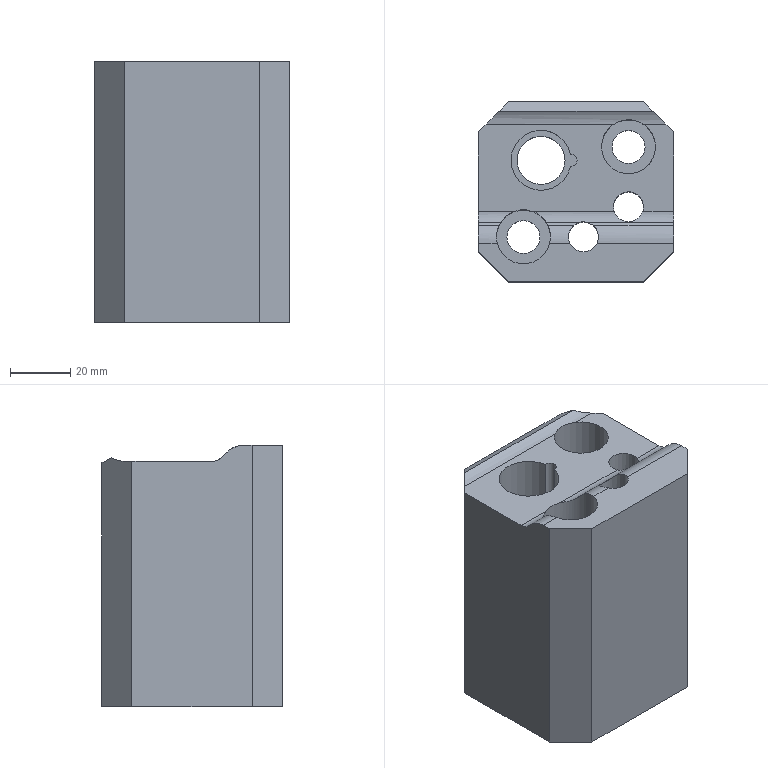Part | NX | features solid 2 | 1 solid | 35 faces | box 65 x 60 x 87.008 mm | volume 234340 mm3 | plane 19 | cylinder 16 | commonest cylinder face diameters 16 x5 10 x4 11 x2 18 x2 4 x1 20 x1
STEP:
#1=CARTESIAN_POINT('',(-255.,-515.,5.));
#2=VERTEX_POINT('',#1);
#3=CARTESIAN_POINT('',(-255.,-515.,92.008));
#4=VERTEX_POINT('',#3);
#5=CARTESIAN_POINT('',(-255.,-515.,10.));
#6=DIRECTION('',(0.,0.,1.));
#7=VECTOR('',#6,1000.);
#8=LINE('',#5,#7);
#9=EDGE_CURVE('',#2,#4,#8,.T.);
#10=ORIENTED_EDGE('',*,*,#9,.T.);
#11=CARTESIAN_POINT('',(-300.,-515.,92.008));
#12=VERTEX_POINT('',#11);
#13=CARTESIAN_POINT('',(-260.,-515.,92.008));
#14=DIRECTION('',(-1.,0.,0.));
#15=VECTOR('',#14,1000.);
#16=LINE('',#13,#15);
#17=EDGE_CURVE('',#4,#12,#16,.T.);
#18=ORIENTED_EDGE('',*,*,#17,.T.);
#19=CARTESIAN_POINT('',(-300.,-515.,5.));
#20=VERTEX_POINT('',#19);
#21=CARTESIAN_POINT('',(-300.,-515.,10.));
#22=DIRECTION('',(0.,0.,-1.));
#23=VECTOR('',#22,1000.);
#24=LINE('',#21,#23);
#25=EDGE_CURVE('',#12,#20,#24,.T.);
#26=ORIENTED_EDGE('',*,*,#25,.T.);
#27=CARTESIAN_POINT('',(-260.,-515.,5.));
#28=DIRECTION('',(1.,0.,0.));
#29=VECTOR('',#28,1000.);
#30=LINE('',#27,#29);
#31=EDGE_CURVE('',#20,#2,#30,.T.);
#32=ORIENTED_EDGE('',*,*,#31,.T.);
#33=EDGE_LOOP('',(#10,#18,#26,#32));
#34=FACE_BOUND('',#33,.T.);
#35=CARTESIAN_POINT('',(-260.,-515.,10.));
#36=DIRECTION('',(0.,-1.,0.));
#37=DIRECTION('',(0.,0.,-1.));
#38=AXIS2_PLACEMENT_3D('',#35,#36,#37);
#39=PLANE('',#38);
#40=ADVANCED_FACE('',(#34),#39,.T.);
#41=CARTESIAN_POINT('',(-310.,-505.,5.));
#42=VERTEX_POINT('',#41);
#43=CARTESIAN_POINT('',(-310.,-505.,92.008));
#44=VERTEX_POINT('',#43);
#45=CARTESIAN_POINT('',(-310.,-505.,10.));
#46=DIRECTION('',(0.,0.,1.));
#47=VECTOR('',#46,1000.);
#48=LINE('',#45,#47);
#49=EDGE_CURVE('',#42,#44,#48,.T.);
#50=ORIENTED_EDGE('',*,*,#49,.T.);
#51=CARTESIAN_POINT('',(-310.,-502.176,92.008));
#52=VERTEX_POINT('',#51);
#53=CARTESIAN_POINT('',(-310.,-505.,92.008));
#54=DIRECTION('',(0.,1.,0.));
#55=VECTOR('',#54,1000.);
#56=LINE('',#53,#55);
#57=EDGE_CURVE('',#44,#52,#56,.T.);
#58=ORIENTED_EDGE('',*,*,#57,.T.);
#59=CARTESIAN_POINT('',(-310.,-496.288,89.423));
#60=VERTEX_POINT('',#59);
#61=CARTESIAN_POINT('',(-310.,-502.176,84.008));
#62=DIRECTION('',(-1.,0.,0.));
#63=DIRECTION('',(0.,0.,1.));
#64=AXIS2_PLACEMENT_3D('',#61,#62,#63);
#65=CIRCLE('',#64,8.);
#66=EDGE_CURVE('',#52,#60,#65,.T.);
#67=ORIENTED_EDGE('',*,*,#66,.T.);
#68=CARTESIAN_POINT('',(-310.,-495.276,88.323));
#69=VERTEX_POINT('',#68);
#70=CARTESIAN_POINT('',(-310.,-460.707,50.738));
#71=DIRECTION('',(0.,0.677,-0.736));
#72=VECTOR('',#71,1000.);
#73=LINE('',#70,#72);
#74=EDGE_CURVE('',#60,#69,#73,.T.);
#75=ORIENTED_EDGE('',*,*,#74,.T.);
#76=CARTESIAN_POINT('',(-310.,-491.596,86.708));
#77=VERTEX_POINT('',#76);
#78=CARTESIAN_POINT('',(-310.,-491.596,91.708));
#79=DIRECTION('',(-1.,0.,0.));
#80=DIRECTION('',(0.,0.,1.));
#81=AXIS2_PLACEMENT_3D('',#78,#79,#80);
#82=CIRCLE('',#81,5.);
#83=EDGE_CURVE('',#77,#69,#82,.T.);
#84=ORIENTED_EDGE('',*,*,#83,.F.);
#85=CARTESIAN_POINT('',(-310.,-465.,86.708));
#86=VERTEX_POINT('',#85);
#87=CARTESIAN_POINT('',(-310.,-505.,86.708));
#88=DIRECTION('',(0.,1.,0.));
#89=VECTOR('',#88,1000.);
#90=LINE('',#87,#89);
#91=EDGE_CURVE('',#77,#86,#90,.T.);
#92=ORIENTED_EDGE('',*,*,#91,.T.);
#93=CARTESIAN_POINT('',(-310.,-465.,5.));
#94=VERTEX_POINT('',#93);
#95=CARTESIAN_POINT('',(-310.,-465.,10.));
#96=DIRECTION('',(0.,0.,-1.));
#97=VECTOR('',#96,1000.);
#98=LINE('',#95,#97);
#99=EDGE_CURVE('',#86,#94,#98,.T.);
#100=ORIENTED_EDGE('',*,*,#99,.T.);
#101=CARTESIAN_POINT('',(-310.,-505.,5.));
#102=DIRECTION('',(0.,-1.,0.));
#103=VECTOR('',#102,1000.);
#104=LINE('',#101,#103);
#105=EDGE_CURVE('',#94,#42,#104,.T.);
#106=ORIENTED_EDGE('',*,*,#105,.T.);
#107=EDGE_LOOP('',(#50,#58,#67,#75,#84,#92,#100,#106));
#108=FACE_BOUND('',#107,.T.);
#109=CARTESIAN_POINT('',(-310.,-505.,10.));
#110=DIRECTION('',(-1.,0.,0.));
#111=DIRECTION('',(0.,0.,1.));
#112=AXIS2_PLACEMENT_3D('',#109,#110,#111);
#113=PLANE('',#112);
#114=ADVANCED_FACE('',(#108),#113,.T.);
#115=CARTESIAN_POINT('',(-300.,-455.,5.));
#116=VERTEX_POINT('',#115);
#117=CARTESIAN_POINT('',(-300.,-455.,86.231));
#118=VERTEX_POINT('',#117);
#119=CARTESIAN_POINT('',(-300.,-455.,10.));
#120=DIRECTION('',(0.,0.,1.));
#121=VECTOR('',#120,1000.);
#122=LINE('',#119,#121);
#123=EDGE_CURVE('',#116,#118,#122,.T.);
#124=ORIENTED_EDGE('',*,*,#123,.T.);
#125=CARTESIAN_POINT('',(-255.,-455.,86.231));
#126=VERTEX_POINT('',#125);
#127=CARTESIAN_POINT('',(-255.,-455.,86.231));
#128=DIRECTION('',(1.,0.,0.));
#129=VECTOR('',#128,1000.);
#130=LINE('',#127,#129);
#131=EDGE_CURVE('',#118,#126,#130,.T.);
#132=ORIENTED_EDGE('',*,*,#131,.T.);
#133=CARTESIAN_POINT('',(-255.,-455.,5.));
#134=VERTEX_POINT('',#133);
#135=CARTESIAN_POINT('',(-255.,-455.,10.));
#136=DIRECTION('',(0.,0.,-1.));
#137=VECTOR('',#136,1000.);
#138=LINE('',#135,#137);
#139=EDGE_CURVE('',#126,#134,#138,.T.);
#140=ORIENTED_EDGE('',*,*,#139,.T.);
#141=CARTESIAN_POINT('',(-260.,-455.,5.));
#142=DIRECTION('',(-1.,0.,0.));
#143=VECTOR('',#142,1000.);
#144=LINE('',#141,#143);
#145=EDGE_CURVE('',#134,#116,#144,.T.);
#146=ORIENTED_EDGE('',*,*,#145,.T.);
#147=EDGE_LOOP('',(#124,#132,#140,#146));
#148=FACE_BOUND('',#147,.T.);
#149=CARTESIAN_POINT('',(-260.,-455.,10.));
#150=DIRECTION('',(0.,1.,0.));
#151=DIRECTION('',(0.,0.,1.));
#152=AXIS2_PLACEMENT_3D('',#149,#150,#151);
#153=PLANE('',#152);
#154=ADVANCED_FACE('',(#148),#153,.T.);
#155=CARTESIAN_POINT('',(-245.,-496.288,89.423));
#156=VERTEX_POINT('',#155);
#157=CARTESIAN_POINT('',(-245.,-502.176,92.008));
#158=VERTEX_POINT('',#157);
#159=CARTESIAN_POINT('',(-245.,-502.176,84.008));
#160=DIRECTION('',(1.,0.,0.));
#161=DIRECTION('',(0.,0.,-1.));
#162=AXIS2_PLACEMENT_3D('',#159,#160,#161);
#163=CIRCLE('',#162,8.);
#164=EDGE_CURVE('',#156,#158,#163,.T.);
#165=ORIENTED_EDGE('',*,*,#164,.T.);
#166=CARTESIAN_POINT('',(-245.,-505.,92.008));
#167=VERTEX_POINT('',#166);
#168=CARTESIAN_POINT('',(-245.,-505.,92.008));
#169=DIRECTION('',(0.,-1.,0.));
#170=VECTOR('',#169,1000.);
#171=LINE('',#168,#170);
#172=EDGE_CURVE('',#158,#167,#171,.T.);
#173=ORIENTED_EDGE('',*,*,#172,.T.);
#174=CARTESIAN_POINT('',(-245.,-505.,5.));
#175=VERTEX_POINT('',#174);
#176=CARTESIAN_POINT('',(-245.,-505.,10.));
#177=DIRECTION('',(0.,0.,-1.));
#178=VECTOR('',#177,1000.);
#179=LINE('',#176,#178);
#180=EDGE_CURVE('',#167,#175,#179,.T.);
#181=ORIENTED_EDGE('',*,*,#180,.T.);
#182=CARTESIAN_POINT('',(-245.,-465.,5.));
#183=VERTEX_POINT('',#182);
#184=CARTESIAN_POINT('',(-245.,-505.,5.));
#185=DIRECTION('',(0.,1.,0.));
#186=VECTOR('',#185,1000.);
#187=LINE('',#184,#186);
#188=EDGE_CURVE('',#175,#183,#187,.T.);
#189=ORIENTED_EDGE('',*,*,#188,.T.);
#190=CARTESIAN_POINT('',(-245.,-465.,86.708));
#191=VERTEX_POINT('',#190);
#192=CARTESIAN_POINT('',(-245.,-465.,10.));
#193=DIRECTION('',(0.,0.,1.));
#194=VECTOR('',#193,1000.);
#195=LINE('',#192,#194);
#196=EDGE_CURVE('',#183,#191,#195,.T.);
#197=ORIENTED_EDGE('',*,*,#196,.T.);
#198=CARTESIAN_POINT('',(-245.,-491.596,86.708));
#199=VERTEX_POINT('',#198);
#200=CARTESIAN_POINT('',(-245.,-505.,86.708));
#201=DIRECTION('',(0.,-1.,0.));
#202=VECTOR('',#201,1000.);
#203=LINE('',#200,#202);
#204=EDGE_CURVE('',#191,#199,#203,.T.);
#205=ORIENTED_EDGE('',*,*,#204,.T.);
#206=CARTESIAN_POINT('',(-245.,-495.276,88.323));
#207=VERTEX_POINT('',#206);
#208=CARTESIAN_POINT('',(-245.,-491.596,91.708));
#209=DIRECTION('',(1.,0.,0.));
#210=DIRECTION('',(0.,0.,-1.));
#211=AXIS2_PLACEMENT_3D('',#208,#209,#210);
#212=CIRCLE('',#211,5.);
#213=EDGE_CURVE('',#207,#199,#212,.T.);
#214=ORIENTED_EDGE('',*,*,#213,.F.);
#215=CARTESIAN_POINT('',(-245.,-460.707,50.738));
#216=DIRECTION('',(0.,-0.677,0.736));
#217=VECTOR('',#216,1000.);
#218=LINE('',#215,#217);
#219=EDGE_CURVE('',#207,#156,#218,.T.);
#220=ORIENTED_EDGE('',*,*,#219,.T.);
#221=EDGE_LOOP('',(#165,#173,#181,#189,#197,#205,#214,#220));
#222=FACE_BOUND('',#221,.T.);
#223=CARTESIAN_POINT('',(-245.,-505.,10.));
#224=DIRECTION('',(1.,0.,0.));
#225=DIRECTION('',(0.,0.,-1.));
#226=AXIS2_PLACEMENT_3D('',#223,#224,#225);
#227=PLANE('',#226);
#228=ADVANCED_FACE('',(#222),#227,.T.);
#229=ORIENTED_EDGE('',*,*,#180,.F.);
#230=CARTESIAN_POINT('',(-255.,-515.,92.008));
#231=DIRECTION('',(0.7071,0.7071,0.));
#232=VECTOR('',#231,1000.);
#233=LINE('',#230,#232);
#234=EDGE_CURVE('',#167,#4,#233,.F.);
#235=ORIENTED_EDGE('',*,*,#234,.T.);
#236=ORIENTED_EDGE('',*,*,#9,.F.);
#237=CARTESIAN_POINT('',(-252.5,-512.5,5.));
#238=DIRECTION('',(0.7071,0.7071,0.));
#239=VECTOR('',#238,1000.);
#240=LINE('',#237,#239);
#241=EDGE_CURVE('',#175,#2,#240,.F.);
#242=ORIENTED_EDGE('',*,*,#241,.F.);
#243=EDGE_LOOP('',(#229,#235,#236,#242));
#244=FACE_BOUND('',#243,.T.);
#245=CARTESIAN_POINT('',(-255.,-515.,10.));
#246=DIRECTION('',(-0.7071,0.7071,0.));
#247=DIRECTION('',(-0.7071,-0.7071,0.));
#248=AXIS2_PLACEMENT_3D('',#245,#246,#247);
#249=PLANE('',#248);
#250=ADVANCED_FACE('',(#244),#249,.F.);
#251=ORIENTED_EDGE('',*,*,#25,.F.);
#252=CARTESIAN_POINT('',(-310.,-505.,92.008));
#253=DIRECTION('',(0.7071,-0.7071,0.));
#254=VECTOR('',#253,1000.);
#255=LINE('',#252,#254);
#256=EDGE_CURVE('',#12,#44,#255,.F.);
#257=ORIENTED_EDGE('',*,*,#256,.T.);
#258=ORIENTED_EDGE('',*,*,#49,.F.);
#259=CARTESIAN_POINT('',(-285.,-530.,5.));
#260=DIRECTION('',(0.7071,-0.7071,0.));
#261=VECTOR('',#260,1000.);
#262=LINE('',#259,#261);
#263=EDGE_CURVE('',#20,#42,#262,.F.);
#264=ORIENTED_EDGE('',*,*,#263,.F.);
#265=EDGE_LOOP('',(#251,#257,#258,#264));
#266=FACE_BOUND('',#265,.T.);
#267=CARTESIAN_POINT('',(-310.,-505.,10.));
#268=DIRECTION('',(0.7071,0.7071,0.));
#269=DIRECTION('',(-0.7071,0.7071,0.));
#270=AXIS2_PLACEMENT_3D('',#267,#268,#269);
#271=PLANE('',#270);
#272=ADVANCED_FACE('',(#266),#271,.F.);
#273=CARTESIAN_POINT('',(-303.154,-458.154,87.961));
#274=VERTEX_POINT('',#273);
#275=CARTESIAN_POINT('',(-307.454,-462.454,86.708));
#276=VERTEX_POINT('',#275);
#277=CARTESIAN_POINT('',(-307.454,-462.454,94.708));
#278=DIRECTION('',(0.7071,-0.7071,0.));
#279=DIRECTION('',(0.7071,0.7071,0.));
#280=AXIS2_PLACEMENT_3D('',#277,#278,#279);
#281=ELLIPSE('',#280,11.314,8.);
#282=EDGE_CURVE('',#274,#276,#281,.F.);
#283=ORIENTED_EDGE('',*,*,#282,.F.);
#284=CARTESIAN_POINT('',(-281.828,-436.828,76.264));
#285=DIRECTION('',(0.6593,0.6593,-0.3616));
#286=VECTOR('',#285,1000.);
#287=LINE('',#284,#286);
#288=EDGE_CURVE('',#274,#118,#287,.T.);
#289=ORIENTED_EDGE('',*,*,#288,.T.);
#290=ORIENTED_EDGE('',*,*,#123,.F.);
#291=CARTESIAN_POINT('',(-305.,-460.,5.));
#292=DIRECTION('',(-0.7071,-0.7071,0.));
#293=VECTOR('',#292,1000.);
#294=LINE('',#291,#293);
#295=EDGE_CURVE('',#94,#116,#294,.F.);
#296=ORIENTED_EDGE('',*,*,#295,.F.);
#297=ORIENTED_EDGE('',*,*,#99,.F.);
#298=CARTESIAN_POINT('',(-300.,-455.,86.708));
#299=DIRECTION('',(-0.7071,-0.7071,0.));
#300=VECTOR('',#299,1000.);
#301=LINE('',#298,#300);
#302=EDGE_CURVE('',#86,#276,#301,.F.);
#303=ORIENTED_EDGE('',*,*,#302,.T.);
#304=EDGE_LOOP('',(#283,#289,#290,#296,#297,#303));
#305=FACE_BOUND('',#304,.T.);
#306=CARTESIAN_POINT('',(-300.,-455.,10.));
#307=DIRECTION('',(0.7071,-0.7071,0.));
#308=DIRECTION('',(0.7071,0.7071,0.));
#309=AXIS2_PLACEMENT_3D('',#306,#307,#308);
#310=PLANE('',#309);
#311=ADVANCED_FACE('',(#305),#310,.F.);
#312=ORIENTED_EDGE('',*,*,#139,.F.);
#313=CARTESIAN_POINT('',(-251.846,-458.154,87.961));
#314=VERTEX_POINT('',#313);
#315=CARTESIAN_POINT('',(-264.48,-445.52,81.032));
#316=DIRECTION('',(0.6593,-0.6593,0.3616));
#317=VECTOR('',#316,1000.);
#318=LINE('',#315,#317);
#319=EDGE_CURVE('',#126,#314,#318,.T.);
#320=ORIENTED_EDGE('',*,*,#319,.T.);
#321=CARTESIAN_POINT('',(-247.546,-462.454,86.708));
#322=VERTEX_POINT('',#321);
#323=CARTESIAN_POINT('',(-247.546,-462.454,94.708));
#324=DIRECTION('',(-0.7071,-0.7071,0.));
#325=DIRECTION('',(0.7071,-0.7071,0.));
#326=AXIS2_PLACEMENT_3D('',#323,#324,#325);
#327=ELLIPSE('',#326,11.314,8.);
#328=EDGE_CURVE('',#322,#314,#327,.F.);
#329=ORIENTED_EDGE('',*,*,#328,.F.);
#330=CARTESIAN_POINT('',(-245.,-465.,86.708));
#331=DIRECTION('',(-0.7071,0.7071,0.));
#332=VECTOR('',#331,1000.);
#333=LINE('',#330,#332);
#334=EDGE_CURVE('',#322,#191,#333,.F.);
#335=ORIENTED_EDGE('',*,*,#334,.T.);
#336=ORIENTED_EDGE('',*,*,#196,.F.);
#337=CARTESIAN_POINT('',(-232.5,-477.5,5.));
#338=DIRECTION('',(-0.7071,0.7071,0.));
#339=VECTOR('',#338,1000.);
#340=LINE('',#337,#339);
#341=EDGE_CURVE('',#134,#183,#340,.F.);
#342=ORIENTED_EDGE('',*,*,#341,.F.);
#343=EDGE_LOOP('',(#312,#320,#329,#335,#336,#342));
#344=FACE_BOUND('',#343,.T.);
#345=CARTESIAN_POINT('',(-245.,-465.,10.));
#346=DIRECTION('',(-0.7071,-0.7071,0.));
#347=DIRECTION('',(0.7071,-0.7071,0.));
#348=AXIS2_PLACEMENT_3D('',#345,#346,#347);
#349=PLANE('',#348);
#350=ADVANCED_FACE('',(#344),#349,.F.);
#351=CARTESIAN_POINT('',(-269.,-470.,35.));
#352=VERTEX_POINT('',#351);
#353=CARTESIAN_POINT('',(-260.,-470.,35.));
#354=DIRECTION('',(0.,0.,-1.));
#355=DIRECTION('',(-1.,0.,0.));
#356=AXIS2_PLACEMENT_3D('',#353,#354,#355);
#357=CIRCLE('',#356,9.);
#358=EDGE_CURVE('',#352,#352,#357,.T.);
#359=ORIENTED_EDGE('',*,*,#358,.T.);
#360=EDGE_LOOP('',(#359));
#361=FACE_BOUND('',#360,.T.);
#362=CARTESIAN_POINT('',(-255.095,-462.454,86.708));
#363=VERTEX_POINT('',#362);
#364=CARTESIAN_POINT('',(-264.905,-462.454,86.708));
#365=VERTEX_POINT('',#364);
#366=CARTESIAN_POINT('',(-260.,-470.,86.708));
#367=DIRECTION('',(0.,0.,1.));
#368=DIRECTION('',(1.,0.,0.));
#369=AXIS2_PLACEMENT_3D('',#366,#367,#368);
#370=CIRCLE('',#369,9.);
#371=EDGE_CURVE('',#363,#365,#370,.F.);
#372=ORIENTED_EDGE('',*,*,#371,.F.);
#373=CARTESIAN_POINT('',(-255.095,-462.454,86.708));
#374=CARTESIAN_POINT('',(-256.558,-461.503,86.708));
#375=CARTESIAN_POINT('',(-259.984,-460.497,86.974));
#376=CARTESIAN_POINT('',(-263.442,-461.503,86.708));
#377=CARTESIAN_POINT('',(-264.905,-462.454,86.708));
#378=B_SPLINE_CURVE_WITH_KNOTS('',3,(#373,#374,#375,#376,#377),.UNSPECIFIED.,.F.,.F.,(4,1,4),(0.,0.00516,0.01032),.UNSPECIFIED.);
#379=EDGE_CURVE('',#363,#365,#378,.T.);
#380=ORIENTED_EDGE('',*,*,#379,.T.);
#381=EDGE_LOOP('',(#372,#380));
#382=FACE_BOUND('',#381,.T.);
#383=CARTESIAN_POINT('',(-260.,-470.,110.));
#384=DIRECTION('',(0.,0.,-1.));
#385=DIRECTION('',(-1.,0.,0.));
#386=AXIS2_PLACEMENT_3D('',#383,#384,#385);
#387=CYLINDRICAL_SURFACE('',#386,9.);
#388=ADVANCED_FACE('',(#361,#382),#387,.F.);
#389=CARTESIAN_POINT('',(-304.,-500.,35.));
#390=VERTEX_POINT('',#389);
#391=CARTESIAN_POINT('',(-295.,-500.,35.));
#392=DIRECTION('',(0.,0.,-1.));
#393=DIRECTION('',(-1.,0.,0.));
#394=AXIS2_PLACEMENT_3D('',#391,#392,#393);
#395=CIRCLE('',#394,9.);
#396=EDGE_CURVE('',#390,#390,#395,.T.);
#397=ORIENTED_EDGE('',*,*,#396,.T.);
#398=EDGE_LOOP('',(#397));
#399=FACE_BOUND('',#398,.T.);
#400=CARTESIAN_POINT('',(-286.801,-496.288,89.423));
#401=VERTEX_POINT('',#400);
#402=CARTESIAN_POINT('',(-286.267,-502.176,92.008));
#403=VERTEX_POINT('',#402);
#404=CARTESIAN_POINT('',(-286.801,-496.288,89.423));
#405=CARTESIAN_POINT('',(-286.47,-497.019,90.218));
#406=CARTESIAN_POINT('',(-285.896,-498.815,91.527));
#407=CARTESIAN_POINT('',(-285.993,-501.076,92.008));
#408=CARTESIAN_POINT('',(-286.267,-502.176,92.008));
#409=B_SPLINE_CURVE_WITH_KNOTS('',3,(#404,#405,#406,#407,#408),.UNSPECIFIED.,.F.,.F.,(4,1,4),(0.,0.00335,0.0067),.UNSPECIFIED.);
#410=EDGE_CURVE('',#401,#403,#409,.T.);
#411=ORIENTED_EDGE('',*,*,#410,.F.);
#412=CARTESIAN_POINT('',(-287.34,-495.276,88.323));
#413=VERTEX_POINT('',#412);
#414=CARTESIAN_POINT('',(-295.,-500.,93.459));
#415=DIRECTION('',(0.,0.736,0.677));
#416=DIRECTION('',(0.,0.677,-0.736));
#417=AXIS2_PLACEMENT_3D('',#414,#415,#416);
#418=ELLIPSE('',#417,13.295,9.);
#419=EDGE_CURVE('',#413,#401,#418,.F.);
#420=ORIENTED_EDGE('',*,*,#419,.F.);
#421=CARTESIAN_POINT('',(-291.78,-491.596,86.708));
#422=VERTEX_POINT('',#421);
#423=CARTESIAN_POINT('',(-287.34,-495.276,88.323));
#424=CARTESIAN_POINT('',(-287.745,-494.619,87.609));
#425=CARTESIAN_POINT('',(-288.986,-493.061,86.771));
#426=CARTESIAN_POINT('',(-290.803,-491.97,86.708));
#427=CARTESIAN_POINT('',(-291.78,-491.596,86.708));
#428=B_SPLINE_CURVE_WITH_KNOTS('',3,(#423,#424,#425,#426,#427),.UNSPECIFIED.,.F.,.F.,(4,1,4),(0.,0.003104,0.006208),.UNSPECIFIED.);
#429=EDGE_CURVE('',#413,#422,#428,.T.);
#430=ORIENTED_EDGE('',*,*,#429,.T.);
#431=CARTESIAN_POINT('',(-298.22,-491.596,86.708));
#432=VERTEX_POINT('',#431);
#433=CARTESIAN_POINT('',(-295.,-500.,86.708));
#434=DIRECTION('',(0.,0.,1.));
#435=DIRECTION('',(1.,0.,0.));
#436=AXIS2_PLACEMENT_3D('',#433,#434,#435);
#437=CIRCLE('',#436,9.);
#438=EDGE_CURVE('',#432,#422,#437,.F.);
#439=ORIENTED_EDGE('',*,*,#438,.F.);
#440=CARTESIAN_POINT('',(-302.66,-495.276,88.323));
#441=VERTEX_POINT('',#440);
#442=CARTESIAN_POINT('',(-298.22,-491.596,86.708));
#443=CARTESIAN_POINT('',(-299.198,-491.97,86.708));
#444=CARTESIAN_POINT('',(-301.015,-493.063,86.772));
#445=CARTESIAN_POINT('',(-302.255,-494.618,87.608));
#446=CARTESIAN_POINT('',(-302.66,-495.276,88.323));
#447=B_SPLINE_CURVE_WITH_KNOTS('',3,(#442,#443,#444,#445,#446),.UNSPECIFIED.,.F.,.F.,(4,1,4),(0.,0.003103,0.006207),.UNSPECIFIED.);
#448=EDGE_CURVE('',#432,#441,#447,.T.);
#449=ORIENTED_EDGE('',*,*,#448,.T.);
#450=CARTESIAN_POINT('',(-303.199,-496.288,89.423));
#451=VERTEX_POINT('',#450);
#452=CARTESIAN_POINT('',(-295.,-500.,93.459));
#453=DIRECTION('',(0.,0.736,0.677));
#454=DIRECTION('',(0.,0.677,-0.736));
#455=AXIS2_PLACEMENT_3D('',#452,#453,#454);
#456=ELLIPSE('',#455,13.295,9.);
#457=EDGE_CURVE('',#451,#441,#456,.F.);
#458=ORIENTED_EDGE('',*,*,#457,.F.);
#459=CARTESIAN_POINT('',(-303.733,-502.176,92.008));
#460=VERTEX_POINT('',#459);
#461=CARTESIAN_POINT('',(-303.733,-502.176,92.008));
#462=CARTESIAN_POINT('',(-304.007,-501.078,92.008));
#463=CARTESIAN_POINT('',(-304.105,-498.822,91.531));
#464=CARTESIAN_POINT('',(-303.53,-497.019,90.218));
#465=CARTESIAN_POINT('',(-303.199,-496.288,89.423));
#466=B_SPLINE_CURVE_WITH_KNOTS('',3,(#461,#462,#463,#464,#465),.UNSPECIFIED.,.F.,.F.,(4,1,4),(0.,0.003343,0.006686),.UNSPECIFIED.);
#467=EDGE_CURVE('',#460,#451,#466,.T.);
#468=ORIENTED_EDGE('',*,*,#467,.F.);
#469=CARTESIAN_POINT('',(-295.,-500.,92.008));
#470=DIRECTION('',(0.,0.,1.));
#471=DIRECTION('',(1.,0.,0.));
#472=AXIS2_PLACEMENT_3D('',#469,#470,#471);
#473=CIRCLE('',#472,9.);
#474=EDGE_CURVE('',#403,#460,#473,.F.);
#475=ORIENTED_EDGE('',*,*,#474,.F.);
#476=EDGE_LOOP('',(#411,#420,#430,#439,#449,#458,#468,#475));
#477=FACE_BOUND('',#476,.T.);
#478=CARTESIAN_POINT('',(-295.,-500.,110.));
#479=DIRECTION('',(0.,0.,-1.));
#480=DIRECTION('',(-1.,0.,0.));
#481=AXIS2_PLACEMENT_3D('',#478,#479,#480);
#482=CYLINDRICAL_SURFACE('',#481,9.);
#483=ADVANCED_FACE('',(#399,#477),#482,.F.);
#484=CARTESIAN_POINT('',(-265.,-490.,5.));
#485=VERTEX_POINT('',#484);
#486=CARTESIAN_POINT('',(-260.,-490.,5.));
#487=DIRECTION('',(0.,0.,-1.));
#488=DIRECTION('',(-1.,0.,0.));
#489=AXIS2_PLACEMENT_3D('',#486,#487,#488);
#490=CIRCLE('',#489,5.);
#491=EDGE_CURVE('',#485,#485,#490,.T.);
#492=ORIENTED_EDGE('',*,*,#491,.T.);
#493=EDGE_LOOP('',(#492));
#494=FACE_BOUND('',#493,.T.);
#495=CARTESIAN_POINT('',(-264.739,-491.596,86.708));
#496=VERTEX_POINT('',#495);
#497=CARTESIAN_POINT('',(-255.261,-491.596,86.708));
#498=VERTEX_POINT('',#497);
#499=CARTESIAN_POINT('',(-260.,-490.,86.708));
#500=DIRECTION('',(0.,0.,1.));
#501=DIRECTION('',(1.,0.,0.));
#502=AXIS2_PLACEMENT_3D('',#499,#500,#501);
#503=CIRCLE('',#502,5.);
#504=EDGE_CURVE('',#496,#498,#503,.F.);
#505=ORIENTED_EDGE('',*,*,#504,.F.);
#506=CARTESIAN_POINT('',(-264.739,-491.596,86.708));
#507=CARTESIAN_POINT('',(-264.394,-492.618,86.708));
#508=CARTESIAN_POINT('',(-263.407,-493.895,87.181));
#509=CARTESIAN_POINT('',(-261.599,-494.824,87.872));
#510=CARTESIAN_POINT('',(-259.457,-495.173,88.22));
#511=CARTESIAN_POINT('',(-256.902,-494.32,87.344));
#512=CARTESIAN_POINT('',(-255.605,-492.617,86.708));
#513=CARTESIAN_POINT('',(-255.261,-491.596,86.708));
#514=B_SPLINE_CURVE_WITH_KNOTS('',3,(#506,#507,#508,#509,#510,#511,#512,#513),.UNSPECIFIED.,.F.,.F.,(4,1,1,1,1,4),(0.,0.003178,0.004767,0.006356,0.009534,0.01271),.UNSPECIFIED.);
#515=EDGE_CURVE('',#496,#498,#514,.T.);
#516=ORIENTED_EDGE('',*,*,#515,.T.);
#517=EDGE_LOOP('',(#505,#516));
#518=FACE_BOUND('',#517,.T.);
#519=CARTESIAN_POINT('',(-260.,-490.,110.));
#520=DIRECTION('',(0.,0.,-1.));
#521=DIRECTION('',(-1.,0.,0.));
#522=AXIS2_PLACEMENT_3D('',#519,#520,#521);
#523=CYLINDRICAL_SURFACE('',#522,5.);
#524=ADVANCED_FACE('',(#494,#518),#523,.F.);
#525=CARTESIAN_POINT('',(-280.,-500.,5.));
#526=VERTEX_POINT('',#525);
#527=CARTESIAN_POINT('',(-275.,-500.,5.));
#528=DIRECTION('',(0.,0.,-1.));
#529=DIRECTION('',(-1.,0.,0.));
#530=AXIS2_PLACEMENT_3D('',#527,#528,#529);
#531=CIRCLE('',#530,5.);
#532=EDGE_CURVE('',#526,#526,#531,.T.);
#533=ORIENTED_EDGE('',*,*,#532,.T.);
#534=EDGE_LOOP('',(#533));
#535=FACE_BOUND('',#534,.T.);
#536=CARTESIAN_POINT('',(-270.498,-502.176,92.008));
#537=VERTEX_POINT('',#536);
#538=CARTESIAN_POINT('',(-279.502,-502.176,92.008));
#539=VERTEX_POINT('',#538);
#540=CARTESIAN_POINT('',(-275.,-500.,92.008));
#541=DIRECTION('',(0.,0.,1.));
#542=DIRECTION('',(1.,0.,0.));
#543=AXIS2_PLACEMENT_3D('',#540,#541,#542);
#544=CIRCLE('',#543,5.);
#545=EDGE_CURVE('',#537,#539,#544,.F.);
#546=ORIENTED_EDGE('',*,*,#545,.F.);
#547=CARTESIAN_POINT('',(-271.65,-496.288,89.423));
#548=VERTEX_POINT('',#547);
#549=CARTESIAN_POINT('',(-271.65,-496.288,89.423));
#550=CARTESIAN_POINT('',(-270.939,-496.93,90.122));
#551=CARTESIAN_POINT('',(-269.822,-498.631,91.478));
#552=CARTESIAN_POINT('',(-269.979,-501.102,92.008));
#553=CARTESIAN_POINT('',(-270.498,-502.176,92.008));
#554=B_SPLINE_CURVE_WITH_KNOTS('',3,(#549,#550,#551,#552,#553),.UNSPECIFIED.,.F.,.F.,(4,1,4),(0.,0.003501,0.007001),.UNSPECIFIED.);
#555=EDGE_CURVE('',#548,#537,#554,.T.);
#556=ORIENTED_EDGE('',*,*,#555,.F.);
#557=CARTESIAN_POINT('',(-273.362,-495.276,88.323));
#558=VERTEX_POINT('',#557);
#559=CARTESIAN_POINT('',(-275.,-500.,93.459));
#560=DIRECTION('',(0.,0.736,0.677));
#561=DIRECTION('',(0.,0.677,-0.736));
#562=AXIS2_PLACEMENT_3D('',#559,#560,#561);
#563=ELLIPSE('',#562,7.386,5.);
#564=EDGE_CURVE('',#558,#548,#563,.F.);
#565=ORIENTED_EDGE('',*,*,#564,.F.);
#566=CARTESIAN_POINT('',(-276.638,-495.276,88.323));
#567=VERTEX_POINT('',#566);
#568=CARTESIAN_POINT('',(-273.362,-495.276,88.323));
#569=CARTESIAN_POINT('',(-274.38,-494.923,87.939));
#570=CARTESIAN_POINT('',(-275.62,-494.923,87.939));
#571=CARTESIAN_POINT('',(-276.638,-495.276,88.323));
#572=B_SPLINE_CURVE_WITH_KNOTS('',3,(#568,#569,#570,#571),.UNSPECIFIED.,.F.,.F.,(4,4),(0.,0.00338),.UNSPECIFIED.);
#573=EDGE_CURVE('',#558,#567,#572,.T.);
#574=ORIENTED_EDGE('',*,*,#573,.T.);
#575=CARTESIAN_POINT('',(-278.35,-496.288,89.423));
#576=VERTEX_POINT('',#575);
#577=CARTESIAN_POINT('',(-275.,-500.,93.459));
#578=DIRECTION('',(0.,0.736,0.677));
#579=DIRECTION('',(0.,0.677,-0.736));
#580=AXIS2_PLACEMENT_3D('',#577,#578,#579);
#581=ELLIPSE('',#580,7.386,5.);
#582=EDGE_CURVE('',#576,#567,#581,.F.);
#583=ORIENTED_EDGE('',*,*,#582,.F.);
#584=CARTESIAN_POINT('',(-279.502,-502.176,92.008));
#585=CARTESIAN_POINT('',(-280.02,-501.105,92.008));
#586=CARTESIAN_POINT('',(-280.182,-498.642,91.484));
#587=CARTESIAN_POINT('',(-279.061,-496.93,90.121));
#588=CARTESIAN_POINT('',(-278.35,-496.288,89.423));
#589=B_SPLINE_CURVE_WITH_KNOTS('',3,(#584,#585,#586,#587,#588),.UNSPECIFIED.,.F.,.F.,(4,1,4),(0.,0.003519,0.007038),.UNSPECIFIED.);
#590=EDGE_CURVE('',#539,#576,#589,.T.);
#591=ORIENTED_EDGE('',*,*,#590,.F.);
#592=EDGE_LOOP('',(#546,#556,#565,#574,#583,#591));
#593=FACE_BOUND('',#592,.T.);
#594=CARTESIAN_POINT('',(-275.,-500.,110.));
#595=DIRECTION('',(0.,0.,-1.));
#596=DIRECTION('',(-1.,0.,0.));
#597=AXIS2_PLACEMENT_3D('',#594,#595,#596);
#598=CYLINDRICAL_SURFACE('',#597,5.);
#599=ADVANCED_FACE('',(#535,#593),#598,.F.);
#600=CARTESIAN_POINT('',(-300.643,-474.5,5.));
#601=VERTEX_POINT('',#600);
#602=CARTESIAN_POINT('',(-289.143,-474.5,5.));
#603=DIRECTION('',(0.,0.,-1.));
#604=DIRECTION('',(-1.,0.,0.));
#605=AXIS2_PLACEMENT_3D('',#602,#603,#604);
#606=CIRCLE('',#605,11.5);
#607=EDGE_CURVE('',#601,#601,#606,.F.);
#608=ORIENTED_EDGE('',*,*,#607,.T.);
#609=EDGE_LOOP('',(#608));
#610=FACE_BOUND('',#609,.T.);
#611=ORIENTED_EDGE('',*,*,#532,.F.);
#612=EDGE_LOOP('',(#611));
#613=FACE_BOUND('',#612,.T.);
#614=ORIENTED_EDGE('',*,*,#491,.F.);
#615=EDGE_LOOP('',(#614));
#616=FACE_BOUND('',#615,.T.);
#617=CARTESIAN_POINT('',(-300.5,-500.,5.));
#618=VERTEX_POINT('',#617);
#619=CARTESIAN_POINT('',(-295.,-500.,5.));
#620=DIRECTION('',(0.,0.,-1.));
#621=DIRECTION('',(-1.,0.,0.));
#622=AXIS2_PLACEMENT_3D('',#619,#620,#621);
#623=CIRCLE('',#622,5.5);
#624=EDGE_CURVE('',#618,#618,#623,.T.);
#625=ORIENTED_EDGE('',*,*,#624,.F.);
#626=EDGE_LOOP('',(#625));
#627=FACE_BOUND('',#626,.T.);
#628=CARTESIAN_POINT('',(-265.5,-470.,5.));
#629=VERTEX_POINT('',#628);
#630=CARTESIAN_POINT('',(-260.,-470.,5.));
#631=DIRECTION('',(0.,0.,-1.));
#632=DIRECTION('',(-1.,0.,0.));
#633=AXIS2_PLACEMENT_3D('',#630,#631,#632);
#634=CIRCLE('',#633,5.5);
#635=EDGE_CURVE('',#629,#629,#634,.T.);
#636=ORIENTED_EDGE('',*,*,#635,.F.);
#637=EDGE_LOOP('',(#636));
#638=FACE_BOUND('',#637,.T.);
#639=ORIENTED_EDGE('',*,*,#188,.F.);
#640=ORIENTED_EDGE('',*,*,#241,.T.);
#641=ORIENTED_EDGE('',*,*,#31,.F.);
#642=ORIENTED_EDGE('',*,*,#263,.T.);
#643=ORIENTED_EDGE('',*,*,#105,.F.);
#644=ORIENTED_EDGE('',*,*,#295,.T.);
#645=ORIENTED_EDGE('',*,*,#145,.F.);
#646=ORIENTED_EDGE('',*,*,#341,.T.);
#647=EDGE_LOOP('',(#639,#640,#641,#642,#643,#644,#645,#646));
#648=FACE_BOUND('',#647,.T.);
#649=CARTESIAN_POINT('',(-260.,-505.,5.));
#650=DIRECTION('',(0.,0.,-1.));
#651=DIRECTION('',(-1.,0.,0.));
#652=AXIS2_PLACEMENT_3D('',#649,#650,#651);
#653=PLANE('',#652);
#654=ADVANCED_FACE('',(#610,#613,#616,#627,#638,#648),#653,.T.);
#655=ORIENTED_EDGE('',*,*,#635,.T.);
#656=EDGE_LOOP('',(#655));
#657=FACE_BOUND('',#656,.T.);
#658=CARTESIAN_POINT('',(-265.5,-470.,35.));
#659=VERTEX_POINT('',#658);
#660=CARTESIAN_POINT('',(-260.,-470.,35.));
#661=DIRECTION('',(0.,0.,-1.));
#662=DIRECTION('',(-1.,0.,0.));
#663=AXIS2_PLACEMENT_3D('',#660,#661,#662);
#664=CIRCLE('',#663,5.5);
#665=EDGE_CURVE('',#659,#659,#664,.T.);
#666=ORIENTED_EDGE('',*,*,#665,.F.);
#667=EDGE_LOOP('',(#666));
#668=FACE_BOUND('',#667,.T.);
#669=CARTESIAN_POINT('',(-260.,-470.,5.));
#670=DIRECTION('',(0.,0.,-1.));
#671=DIRECTION('',(-1.,0.,0.));
#672=AXIS2_PLACEMENT_3D('',#669,#670,#671);
#673=CYLINDRICAL_SURFACE('',#672,5.5);
#674=ADVANCED_FACE('',(#657,#668),#673,.F.);
#675=ORIENTED_EDGE('',*,*,#665,.T.);
#676=EDGE_LOOP('',(#675));
#677=FACE_BOUND('',#676,.T.);
#678=ORIENTED_EDGE('',*,*,#358,.F.);
#679=EDGE_LOOP('',(#678));
#680=FACE_BOUND('',#679,.T.);
#681=CARTESIAN_POINT('',(-260.,-470.,35.));
#682=DIRECTION('',(0.,0.,-1.));
#683=DIRECTION('',(-1.,0.,0.));
#684=AXIS2_PLACEMENT_3D('',#681,#682,#683);
#685=PLANE('',#684);
#686=ADVANCED_FACE('',(#677,#680),#685,.F.);
#687=ORIENTED_EDGE('',*,*,#624,.T.);
#688=EDGE_LOOP('',(#687));
#689=FACE_BOUND('',#688,.T.);
#690=CARTESIAN_POINT('',(-300.5,-500.,35.));
#691=VERTEX_POINT('',#690);
#692=CARTESIAN_POINT('',(-295.,-500.,35.));
#693=DIRECTION('',(0.,0.,-1.));
#694=DIRECTION('',(-1.,0.,0.));
#695=AXIS2_PLACEMENT_3D('',#692,#693,#694);
#696=CIRCLE('',#695,5.5);
#697=EDGE_CURVE('',#691,#691,#696,.T.);
#698=ORIENTED_EDGE('',*,*,#697,.F.);
#699=EDGE_LOOP('',(#698));
#700=FACE_BOUND('',#699,.T.);
#701=CARTESIAN_POINT('',(-295.,-500.,5.));
#702=DIRECTION('',(0.,0.,-1.));
#703=DIRECTION('',(-1.,0.,0.));
#704=AXIS2_PLACEMENT_3D('',#701,#702,#703);
#705=CYLINDRICAL_SURFACE('',#704,5.5);
#706=ADVANCED_FACE('',(#689,#700),#705,.F.);
#707=ORIENTED_EDGE('',*,*,#697,.T.);
#708=EDGE_LOOP('',(#707));
#709=FACE_BOUND('',#708,.T.);
#710=ORIENTED_EDGE('',*,*,#396,.F.);
#711=EDGE_LOOP('',(#710));
#712=FACE_BOUND('',#711,.T.);
#713=CARTESIAN_POINT('',(-295.,-500.,35.));
#714=DIRECTION('',(0.,0.,-1.));
#715=DIRECTION('',(-1.,0.,0.));
#716=AXIS2_PLACEMENT_3D('',#713,#714,#715);
#717=PLANE('',#716);
#718=ADVANCED_FACE('',(#709,#712),#717,.F.);
#719=ORIENTED_EDGE('',*,*,#328,.T.);
#720=CARTESIAN_POINT('',(-6000414.,-458.154,87.961));
#721=DIRECTION('',(1.,0.,0.));
#722=VECTOR('',#721,1000.);
#723=LINE('',#720,#722);
#724=EDGE_CURVE('',#314,#274,#723,.F.);
#725=ORIENTED_EDGE('',*,*,#724,.T.);
#726=ORIENTED_EDGE('',*,*,#282,.T.);
#727=CARTESIAN_POINT('',(-264.905,-462.454,86.708));
#728=CARTESIAN_POINT('',(-279.088,-462.454,86.708));
#729=CARTESIAN_POINT('',(-293.271,-462.454,86.708));
#730=CARTESIAN_POINT('',(-307.454,-462.454,86.708));
#731=B_SPLINE_CURVE_WITH_KNOTS('',3,(#727,#728,#729,#730),.UNSPECIFIED.,.F.,.F.,(4,4),(0.8199,0.8713),.UNSPECIFIED.);
#732=EDGE_CURVE('',#365,#276,#731,.T.);
#733=ORIENTED_EDGE('',*,*,#732,.F.);
#734=ORIENTED_EDGE('',*,*,#379,.F.);
#735=CARTESIAN_POINT('',(-247.546,-462.454,86.708));
#736=CARTESIAN_POINT('',(-250.062,-462.454,86.708));
#737=CARTESIAN_POINT('',(-252.579,-462.454,86.708));
#738=CARTESIAN_POINT('',(-255.095,-462.454,86.708));
#739=B_SPLINE_CURVE_WITH_KNOTS('',3,(#735,#736,#737,#738),.UNSPECIFIED.,.F.,.F.,(4,4),(0.7989,0.808),.UNSPECIFIED.);
#740=EDGE_CURVE('',#322,#363,#739,.T.);
#741=ORIENTED_EDGE('',*,*,#740,.F.);
#742=EDGE_LOOP('',(#719,#725,#726,#733,#734,#741));
#743=FACE_BOUND('',#742,.T.);
#744=CARTESIAN_POINT('',(-6000414.,-462.454,94.708));
#745=DIRECTION('',(1.,0.,0.));
#746=DIRECTION('',(0.,0.,1.));
#747=AXIS2_PLACEMENT_3D('',#744,#745,#746);
#748=CYLINDRICAL_SURFACE('',#747,8.);
#749=ADVANCED_FACE('',(#743),#748,.F.);
#750=CARTESIAN_POINT('',(-279.343,-476.49,86.708));
#751=VERTEX_POINT('',#750);
#752=CARTESIAN_POINT('',(-279.343,-472.51,86.708));
#753=VERTEX_POINT('',#752);
#754=CARTESIAN_POINT('',(-279.143,-474.5,86.708));
#755=DIRECTION('',(0.,0.,1.));
#756=DIRECTION('',(1.,0.,0.));
#757=AXIS2_PLACEMENT_3D('',#754,#755,#756);
#758=CIRCLE('',#757,2.);
#759=EDGE_CURVE('',#751,#753,#758,.T.);
#760=ORIENTED_EDGE('',*,*,#759,.F.);
#761=CARTESIAN_POINT('',(-289.143,-474.5,86.708));
#762=DIRECTION('',(0.,0.,1.));
#763=DIRECTION('',(1.,0.,0.));
#764=AXIS2_PLACEMENT_3D('',#761,#762,#763);
#765=CIRCLE('',#764,10.);
#766=EDGE_CURVE('',#751,#753,#765,.F.);
#767=ORIENTED_EDGE('',*,*,#766,.T.);
#768=EDGE_LOOP('',(#760,#767));
#769=FACE_BOUND('',#768,.T.);
#770=ORIENTED_EDGE('',*,*,#91,.F.);
#771=CARTESIAN_POINT('',(-310.,-491.596,86.708));
#772=CARTESIAN_POINT('',(-306.073,-491.596,86.708));
#773=CARTESIAN_POINT('',(-302.147,-491.596,86.708));
#774=CARTESIAN_POINT('',(-298.22,-491.596,86.708));
#775=B_SPLINE_CURVE_WITH_KNOTS('',3,(#771,#772,#773,#774),.UNSPECIFIED.,.F.,.F.,(4,4),(0.1257,0.1399),.UNSPECIFIED.);
#776=EDGE_CURVE('',#77,#432,#775,.T.);
#777=ORIENTED_EDGE('',*,*,#776,.T.);
#778=ORIENTED_EDGE('',*,*,#438,.T.);
#779=CARTESIAN_POINT('',(-291.78,-491.596,86.708));
#780=CARTESIAN_POINT('',(-282.766,-491.596,86.708));
#781=CARTESIAN_POINT('',(-273.752,-491.596,86.708));
#782=CARTESIAN_POINT('',(-264.739,-491.596,86.708));
#783=B_SPLINE_CURVE_WITH_KNOTS('',3,(#779,#780,#781,#782),.UNSPECIFIED.,.F.,.F.,(4,4),(0.1477,0.1803),.UNSPECIFIED.);
#784=EDGE_CURVE('',#422,#496,#783,.T.);
#785=ORIENTED_EDGE('',*,*,#784,.T.);
#786=ORIENTED_EDGE('',*,*,#504,.T.);
#787=CARTESIAN_POINT('',(-255.261,-491.596,86.708));
#788=CARTESIAN_POINT('',(-251.841,-491.596,86.708));
#789=CARTESIAN_POINT('',(-248.42,-491.596,86.708));
#790=CARTESIAN_POINT('',(-245.,-491.596,86.708));
#791=B_SPLINE_CURVE_WITH_KNOTS('',3,(#787,#788,#789,#790),.UNSPECIFIED.,.F.,.F.,(4,4),(0.1918,0.2042),.UNSPECIFIED.);
#792=EDGE_CURVE('',#498,#199,#791,.T.);
#793=ORIENTED_EDGE('',*,*,#792,.T.);
#794=ORIENTED_EDGE('',*,*,#204,.F.);
#795=ORIENTED_EDGE('',*,*,#334,.F.);
#796=ORIENTED_EDGE('',*,*,#740,.T.);
#797=ORIENTED_EDGE('',*,*,#371,.T.);
#798=ORIENTED_EDGE('',*,*,#732,.T.);
#799=ORIENTED_EDGE('',*,*,#302,.F.);
#800=EDGE_LOOP('',(#770,#777,#778,#785,#786,#793,#794,#795,#796,#797,#798,#799));
#801=FACE_BOUND('',#800,.T.);
#802=CARTESIAN_POINT('',(426.488,227.578,86.708));
#803=DIRECTION('',(0.,0.,1.));
#804=DIRECTION('',(0.,-1.,0.));
#805=AXIS2_PLACEMENT_3D('',#802,#803,#804);
#806=PLANE('',#805);
#807=ADVANCED_FACE('',(#769,#801),#806,.T.);
#808=ORIENTED_EDGE('',*,*,#172,.F.);
#809=CARTESIAN_POINT('',(-245.,-502.176,92.008));
#810=CARTESIAN_POINT('',(-253.499,-502.176,92.008));
#811=CARTESIAN_POINT('',(-261.999,-502.176,92.008));
#812=CARTESIAN_POINT('',(-270.498,-502.176,92.008));
#813=B_SPLINE_CURVE_WITH_KNOTS('',3,(#809,#810,#811,#812),.UNSPECIFIED.,.F.,.F.,(4,4),(0.7958,0.8266),.UNSPECIFIED.);
#814=EDGE_CURVE('',#158,#537,#813,.T.);
#815=ORIENTED_EDGE('',*,*,#814,.T.);
#816=ORIENTED_EDGE('',*,*,#545,.T.);
#817=CARTESIAN_POINT('',(-279.502,-502.176,92.008));
#818=CARTESIAN_POINT('',(-281.757,-502.176,92.008));
#819=CARTESIAN_POINT('',(-284.012,-502.176,92.008));
#820=CARTESIAN_POINT('',(-286.267,-502.176,92.008));
#821=B_SPLINE_CURVE_WITH_KNOTS('',3,(#817,#818,#819,#820),.UNSPECIFIED.,.F.,.F.,(4,4),(0.8375,0.8457),.UNSPECIFIED.);
#822=EDGE_CURVE('',#539,#403,#821,.T.);
#823=ORIENTED_EDGE('',*,*,#822,.T.);
#824=ORIENTED_EDGE('',*,*,#474,.T.);
#825=CARTESIAN_POINT('',(-303.733,-502.176,92.008));
#826=CARTESIAN_POINT('',(-305.822,-502.176,92.008));
#827=CARTESIAN_POINT('',(-307.911,-502.176,92.008));
#828=CARTESIAN_POINT('',(-310.,-502.176,92.008));
#829=B_SPLINE_CURVE_WITH_KNOTS('',3,(#825,#826,#827,#828),.UNSPECIFIED.,.F.,.F.,(4,4),(0.8668,0.8743),.UNSPECIFIED.);
#830=EDGE_CURVE('',#460,#52,#829,.T.);
#831=ORIENTED_EDGE('',*,*,#830,.T.);
#832=ORIENTED_EDGE('',*,*,#57,.F.);
#833=ORIENTED_EDGE('',*,*,#256,.F.);
#834=ORIENTED_EDGE('',*,*,#17,.F.);
#835=ORIENTED_EDGE('',*,*,#234,.F.);
#836=EDGE_LOOP('',(#808,#815,#816,#823,#824,#831,#832,#833,#834,#835));
#837=FACE_BOUND('',#836,.T.);
#838=CARTESIAN_POINT('',(575.068,183.357,92.008));
#839=DIRECTION('',(0.,0.,1.));
#840=DIRECTION('',(0.,-1.,0.));
#841=AXIS2_PLACEMENT_3D('',#838,#839,#840);
#842=PLANE('',#841);
#843=ADVANCED_FACE('',(#837),#842,.T.);
#844=CARTESIAN_POINT('',(-286.801,-496.288,89.423));
#845=CARTESIAN_POINT('',(-283.984,-496.288,89.423));
#846=CARTESIAN_POINT('',(-281.167,-496.288,89.423));
#847=CARTESIAN_POINT('',(-278.35,-496.288,89.423));
#848=B_SPLINE_CURVE_WITH_KNOTS('',3,(#844,#845,#846,#847),.UNSPECIFIED.,.F.,.F.,(4,4),(0.1537,0.1639),.UNSPECIFIED.);
#849=EDGE_CURVE('',#401,#576,#848,.T.);
#850=ORIENTED_EDGE('',*,*,#849,.F.);
#851=ORIENTED_EDGE('',*,*,#410,.T.);
#852=ORIENTED_EDGE('',*,*,#822,.F.);
#853=ORIENTED_EDGE('',*,*,#590,.T.);
#854=EDGE_LOOP('',(#850,#851,#852,#853));
#855=FACE_BOUND('',#854,.T.);
#856=CARTESIAN_POINT('',(6000413.634,-502.176,84.008));
#857=DIRECTION('',(-1.,0.,0.));
#858=DIRECTION('',(0.,0.,-1.));
#859=AXIS2_PLACEMENT_3D('',#856,#857,#858);
#860=CYLINDRICAL_SURFACE('',#859,8.);
#861=ADVANCED_FACE('',(#855),#860,.T.);
#862=ORIENTED_EDGE('',*,*,#66,.F.);
#863=ORIENTED_EDGE('',*,*,#830,.F.);
#864=ORIENTED_EDGE('',*,*,#467,.T.);
#865=CARTESIAN_POINT('',(-310.,-496.288,89.423));
#866=CARTESIAN_POINT('',(-307.733,-496.288,89.423));
#867=CARTESIAN_POINT('',(-305.466,-496.288,89.423));
#868=CARTESIAN_POINT('',(-303.199,-496.288,89.423));
#869=B_SPLINE_CURVE_WITH_KNOTS('',3,(#865,#866,#867,#868),.UNSPECIFIED.,.F.,.F.,(4,4),(0.1257,0.1339),.UNSPECIFIED.);
#870=EDGE_CURVE('',#60,#451,#869,.T.);
#871=ORIENTED_EDGE('',*,*,#870,.F.);
#872=EDGE_LOOP('',(#862,#863,#864,#871));
#873=FACE_BOUND('',#872,.T.);
#874=CARTESIAN_POINT('',(6000413.634,-502.176,84.008));
#875=DIRECTION('',(-1.,0.,0.));
#876=DIRECTION('',(0.,0.,-1.));
#877=AXIS2_PLACEMENT_3D('',#874,#875,#876);
#878=CYLINDRICAL_SURFACE('',#877,8.);
#879=ADVANCED_FACE('',(#873),#878,.T.);
#880=ORIENTED_EDGE('',*,*,#164,.F.);
#881=CARTESIAN_POINT('',(-271.65,-496.288,89.423));
#882=CARTESIAN_POINT('',(-262.767,-496.288,89.423));
#883=CARTESIAN_POINT('',(-253.883,-496.288,89.423));
#884=CARTESIAN_POINT('',(-245.,-496.288,89.423));
#885=B_SPLINE_CURVE_WITH_KNOTS('',3,(#881,#882,#883,#884),.UNSPECIFIED.,.F.,.F.,(4,4),(0.172,0.2042),.UNSPECIFIED.);
#886=EDGE_CURVE('',#548,#156,#885,.T.);
#887=ORIENTED_EDGE('',*,*,#886,.F.);
#888=ORIENTED_EDGE('',*,*,#555,.T.);
#889=ORIENTED_EDGE('',*,*,#814,.F.);
#890=EDGE_LOOP('',(#880,#887,#888,#889));
#891=FACE_BOUND('',#890,.T.);
#892=CARTESIAN_POINT('',(6000413.634,-502.176,84.008));
#893=DIRECTION('',(-1.,0.,0.));
#894=DIRECTION('',(0.,0.,-1.));
#895=AXIS2_PLACEMENT_3D('',#892,#893,#894);
#896=CYLINDRICAL_SURFACE('',#895,8.);
#897=ADVANCED_FACE('',(#891),#896,.T.);
#898=CARTESIAN_POINT('',(-276.638,-495.276,88.323));
#899=CARTESIAN_POINT('',(-280.205,-495.276,88.323));
#900=CARTESIAN_POINT('',(-283.772,-495.276,88.323));
#901=CARTESIAN_POINT('',(-287.34,-495.276,88.323));
#902=B_SPLINE_CURVE_WITH_KNOTS('',3,(#898,#899,#900,#901),.UNSPECIFIED.,.F.,.F.,(4,4),(0.834,0.847),.UNSPECIFIED.);
#903=EDGE_CURVE('',#567,#413,#902,.T.);
#904=ORIENTED_EDGE('',*,*,#903,.T.);
#905=ORIENTED_EDGE('',*,*,#419,.T.);
#906=ORIENTED_EDGE('',*,*,#849,.T.);
#907=ORIENTED_EDGE('',*,*,#582,.T.);
#908=EDGE_LOOP('',(#904,#905,#906,#907));
#909=FACE_BOUND('',#908,.T.);
#910=CARTESIAN_POINT('',(-513.463,-424.358,11.217));
#911=DIRECTION('',(0.,0.736,0.677));
#912=DIRECTION('',(0.,-0.677,0.736));
#913=AXIS2_PLACEMENT_3D('',#910,#911,#912);
#914=PLANE('',#913);
#915=ADVANCED_FACE('',(#909),#914,.T.);
#916=ORIENTED_EDGE('',*,*,#74,.F.);
#917=ORIENTED_EDGE('',*,*,#870,.T.);
#918=ORIENTED_EDGE('',*,*,#457,.T.);
#919=CARTESIAN_POINT('',(-302.66,-495.276,88.323));
#920=CARTESIAN_POINT('',(-305.107,-495.276,88.323));
#921=CARTESIAN_POINT('',(-307.553,-495.276,88.323));
#922=CARTESIAN_POINT('',(-310.,-495.276,88.323));
#923=B_SPLINE_CURVE_WITH_KNOTS('',3,(#919,#920,#921,#922),.UNSPECIFIED.,.F.,.F.,(4,4),(0.8655,0.8743),.UNSPECIFIED.);
#924=EDGE_CURVE('',#441,#69,#923,.T.);
#925=ORIENTED_EDGE('',*,*,#924,.T.);
#926=EDGE_LOOP('',(#916,#917,#918,#925));
#927=FACE_BOUND('',#926,.T.);
#928=CARTESIAN_POINT('',(-513.463,-424.358,11.217));
#929=DIRECTION('',(0.,0.736,0.677));
#930=DIRECTION('',(0.,-0.677,0.736));
#931=AXIS2_PLACEMENT_3D('',#928,#929,#930);
#932=PLANE('',#931);
#933=ADVANCED_FACE('',(#927),#932,.T.);
#934=ORIENTED_EDGE('',*,*,#219,.F.);
#935=CARTESIAN_POINT('',(-245.,-495.276,88.323));
#936=CARTESIAN_POINT('',(-254.454,-495.276,88.323));
#937=CARTESIAN_POINT('',(-263.908,-495.276,88.323));
#938=CARTESIAN_POINT('',(-273.362,-495.276,88.323));
#939=B_SPLINE_CURVE_WITH_KNOTS('',3,(#935,#936,#937,#938),.UNSPECIFIED.,.F.,.F.,(4,4),(0.7958,0.8301),.UNSPECIFIED.);
#940=EDGE_CURVE('',#207,#558,#939,.T.);
#941=ORIENTED_EDGE('',*,*,#940,.T.);
#942=ORIENTED_EDGE('',*,*,#564,.T.);
#943=ORIENTED_EDGE('',*,*,#886,.T.);
#944=EDGE_LOOP('',(#934,#941,#942,#943));
#945=FACE_BOUND('',#944,.T.);
#946=CARTESIAN_POINT('',(-513.463,-424.358,11.217));
#947=DIRECTION('',(0.,0.736,0.677));
#948=DIRECTION('',(0.,-0.677,0.736));
#949=AXIS2_PLACEMENT_3D('',#946,#947,#948);
#950=PLANE('',#949);
#951=ADVANCED_FACE('',(#945),#950,.T.);
#952=ORIENTED_EDGE('',*,*,#940,.F.);
#953=ORIENTED_EDGE('',*,*,#213,.T.);
#954=ORIENTED_EDGE('',*,*,#792,.F.);
#955=ORIENTED_EDGE('',*,*,#515,.F.);
#956=ORIENTED_EDGE('',*,*,#784,.F.);
#957=ORIENTED_EDGE('',*,*,#429,.F.);
#958=ORIENTED_EDGE('',*,*,#903,.F.);
#959=ORIENTED_EDGE('',*,*,#573,.F.);
#960=EDGE_LOOP('',(#952,#953,#954,#955,#956,#957,#958,#959));
#961=FACE_BOUND('',#960,.T.);
#962=CARTESIAN_POINT('',(6000413.634,-491.596,91.708));
#963=DIRECTION('',(-1.,0.,0.));
#964=DIRECTION('',(0.,0.,-1.));
#965=AXIS2_PLACEMENT_3D('',#962,#963,#964);
#966=CYLINDRICAL_SURFACE('',#965,5.);
#967=ADVANCED_FACE('',(#961),#966,.F.);
#968=ORIENTED_EDGE('',*,*,#776,.F.);
#969=ORIENTED_EDGE('',*,*,#83,.T.);
#970=ORIENTED_EDGE('',*,*,#924,.F.);
#971=ORIENTED_EDGE('',*,*,#448,.F.);
#972=EDGE_LOOP('',(#968,#969,#970,#971));
#973=FACE_BOUND('',#972,.T.);
#974=CARTESIAN_POINT('',(6000413.634,-491.596,91.708));
#975=DIRECTION('',(-1.,0.,0.));
#976=DIRECTION('',(0.,0.,-1.));
#977=AXIS2_PLACEMENT_3D('',#974,#975,#976);
#978=CYLINDRICAL_SURFACE('',#977,5.);
#979=ADVANCED_FACE('',(#973),#978,.F.);
#980=ORIENTED_EDGE('',*,*,#607,.F.);
#981=EDGE_LOOP('',(#980));
#982=FACE_BOUND('',#981,.T.);
#983=CARTESIAN_POINT('',(-277.643,-474.5,47.));
#984=VERTEX_POINT('',#983);
#985=CARTESIAN_POINT('',(-289.143,-474.5,47.));
#986=DIRECTION('',(0.,0.,1.));
#987=DIRECTION('',(1.,0.,0.));
#988=AXIS2_PLACEMENT_3D('',#985,#986,#987);
#989=CIRCLE('',#988,11.5);
#990=EDGE_CURVE('',#984,#984,#989,.T.);
#991=ORIENTED_EDGE('',*,*,#990,.T.);
#992=EDGE_LOOP('',(#991));
#993=FACE_BOUND('',#992,.T.);
#994=CARTESIAN_POINT('',(-289.143,-474.5,-13.));
#995=DIRECTION('',(0.,0.,1.));
#996=DIRECTION('',(1.,0.,0.));
#997=AXIS2_PLACEMENT_3D('',#994,#995,#996);
#998=CYLINDRICAL_SURFACE('',#997,11.5);
#999=ADVANCED_FACE('',(#982,#993),#998,.F.);
#1000=CARTESIAN_POINT('',(-281.143,-474.5,47.));
#1001=VERTEX_POINT('',#1000);
#1002=CARTESIAN_POINT('',(-289.143,-474.5,47.));
#1003=DIRECTION('',(0.,0.,1.));
#1004=DIRECTION('',(1.,0.,0.));
#1005=AXIS2_PLACEMENT_3D('',#1002,#1003,#1004);
#1006=CIRCLE('',#1005,8.);
#1007=EDGE_CURVE('',#1001,#1001,#1006,.T.);
#1008=ORIENTED_EDGE('',*,*,#1007,.T.);
#1009=EDGE_LOOP('',(#1008));
#1010=FACE_BOUND('',#1009,.T.);
#1011=ORIENTED_EDGE('',*,*,#990,.F.);
#1012=EDGE_LOOP('',(#1011));
#1013=FACE_BOUND('',#1012,.T.);
#1014=CARTESIAN_POINT('',(-289.143,-474.5,47.));
#1015=DIRECTION('',(0.,0.,1.));
#1016=DIRECTION('',(1.,0.,0.));
#1017=AXIS2_PLACEMENT_3D('',#1014,#1015,#1016);
#1018=PLANE('',#1017);
#1019=ADVANCED_FACE('',(#1010,#1013),#1018,.F.);
#1020=CARTESIAN_POINT('',(-281.143,-474.5,67.));
#1021=VERTEX_POINT('',#1020);
#1022=CARTESIAN_POINT('',(-289.143,-474.5,67.));
#1023=DIRECTION('',(0.,0.,1.));
#1024=DIRECTION('',(1.,0.,0.));
#1025=AXIS2_PLACEMENT_3D('',#1022,#1023,#1024);
#1026=CIRCLE('',#1025,8.);
#1027=EDGE_CURVE('',#1021,#1021,#1026,.T.);
#1028=ORIENTED_EDGE('',*,*,#1027,.T.);
#1029=EDGE_LOOP('',(#1028));
#1030=FACE_BOUND('',#1029,.T.);
#1031=ORIENTED_EDGE('',*,*,#1007,.F.);
#1032=EDGE_LOOP('',(#1031));
#1033=FACE_BOUND('',#1032,.T.);
#1034=CARTESIAN_POINT('',(-289.143,-474.5,17.));
#1035=DIRECTION('',(0.,0.,1.));
#1036=DIRECTION('',(1.,0.,0.));
#1037=AXIS2_PLACEMENT_3D('',#1034,#1035,#1036);
#1038=CYLINDRICAL_SURFACE('',#1037,8.);
#1039=ADVANCED_FACE('',(#1030,#1033),#1038,.F.);
#1040=CARTESIAN_POINT('',(-279.343,-476.49,67.));
#1041=VERTEX_POINT('',#1040);
#1042=CARTESIAN_POINT('',(-279.343,-476.49,267.));
#1043=DIRECTION('',(0.,0.,-1.));
#1044=VECTOR('',#1043,1000.);
#1045=LINE('',#1042,#1044);
#1046=EDGE_CURVE('',#751,#1041,#1045,.T.);
#1047=ORIENTED_EDGE('',*,*,#1046,.T.);
#1048=CARTESIAN_POINT('',(-279.343,-472.51,67.));
#1049=VERTEX_POINT('',#1048);
#1050=CARTESIAN_POINT('',(-289.143,-474.5,67.));
#1051=DIRECTION('',(0.,0.,1.));
#1052=DIRECTION('',(1.,0.,0.));
#1053=AXIS2_PLACEMENT_3D('',#1050,#1051,#1052);
#1054=CIRCLE('',#1053,10.);
#1055=EDGE_CURVE('',#1049,#1041,#1054,.T.);
#1056=ORIENTED_EDGE('',*,*,#1055,.F.);
#1057=CARTESIAN_POINT('',(-279.343,-472.51,267.));
#1058=DIRECTION('',(0.,0.,-1.));
#1059=VECTOR('',#1058,1000.);
#1060=LINE('',#1057,#1059);
#1061=EDGE_CURVE('',#1049,#753,#1060,.F.);
#1062=ORIENTED_EDGE('',*,*,#1061,.T.);
#1063=ORIENTED_EDGE('',*,*,#766,.F.);
#1064=EDGE_LOOP('',(#1047,#1056,#1062,#1063));
#1065=FACE_BOUND('',#1064,.T.);
#1066=CARTESIAN_POINT('',(-289.143,-474.5,267.));
#1067=DIRECTION('',(0.,0.,-1.));
#1068=DIRECTION('',(-1.,0.,0.));
#1069=AXIS2_PLACEMENT_3D('',#1066,#1067,#1068);
#1070=CYLINDRICAL_SURFACE('',#1069,10.);
#1071=ADVANCED_FACE('',(#1065),#1070,.F.);
#1072=ORIENTED_EDGE('',*,*,#1027,.F.);
#1073=EDGE_LOOP('',(#1072));
#1074=FACE_BOUND('',#1073,.T.);
#1075=CARTESIAN_POINT('',(-279.143,-474.5,67.));
#1076=DIRECTION('',(0.,0.,1.));
#1077=DIRECTION('',(1.,0.,0.));
#1078=AXIS2_PLACEMENT_3D('',#1075,#1076,#1077);
#1079=CIRCLE('',#1078,2.);
#1080=EDGE_CURVE('',#1041,#1049,#1079,.T.);
#1081=ORIENTED_EDGE('',*,*,#1080,.T.);
#1082=ORIENTED_EDGE('',*,*,#1055,.T.);
#1083=EDGE_LOOP('',(#1081,#1082));
#1084=FACE_BOUND('',#1083,.T.);
#1085=CARTESIAN_POINT('',(-284.143,-474.5,67.));
#1086=DIRECTION('',(0.,0.,1.));
#1087=DIRECTION('',(1.,0.,0.));
#1088=AXIS2_PLACEMENT_3D('',#1085,#1086,#1087);
#1089=PLANE('',#1088);
#1090=ADVANCED_FACE('',(#1074,#1084),#1089,.T.);
#1091=ORIENTED_EDGE('',*,*,#1046,.F.);
#1092=ORIENTED_EDGE('',*,*,#759,.T.);
#1093=ORIENTED_EDGE('',*,*,#1061,.F.);
#1094=ORIENTED_EDGE('',*,*,#1080,.F.);
#1095=EDGE_LOOP('',(#1091,#1092,#1093,#1094));
#1096=FACE_BOUND('',#1095,.T.);
#1097=CARTESIAN_POINT('',(-279.143,-474.5,67.));
#1098=DIRECTION('',(0.,0.,1.));
#1099=DIRECTION('',(1.,0.,0.));
#1100=AXIS2_PLACEMENT_3D('',#1097,#1098,#1099);
#1101=CYLINDRICAL_SURFACE('',#1100,2.);
#1102=ADVANCED_FACE('',(#1096),#1101,.F.);
#1103=ORIENTED_EDGE('',*,*,#288,.F.);
#1104=ORIENTED_EDGE('',*,*,#724,.F.);
#1105=ORIENTED_EDGE('',*,*,#319,.F.);
#1106=ORIENTED_EDGE('',*,*,#131,.F.);
#1107=EDGE_LOOP('',(#1103,#1104,#1105,#1106));
#1108=FACE_BOUND('',#1107,.T.);
#1109=CARTESIAN_POINT('',(-6000414.,-455.,86.231));
#1110=DIRECTION('',(0.,-0.4809,-0.8768));
#1111=DIRECTION('',(0.,0.8768,-0.4809));
#1112=AXIS2_PLACEMENT_3D('',#1109,#1110,#1111);
#1113=PLANE('',#1112);
#1114=ADVANCED_FACE('',(#1108),#1113,.F.);
#1115=CLOSED_SHELL('',(#40,#114,#154,#228,#250,#272,#311,#350,#388,#483,#524,#599,#654,#674,#686,#706,#718,#749,#807,#843,#861,#879,#897,#915,#933,#951,#967,#979,#999,#1019,#1039,#1071,#1090,#1102,#1114));
#1116=MANIFOLD_SOLID_BREP('',#1115);
#1117=(LENGTH_UNIT()NAMED_UNIT(*)SI_UNIT(.MILLI.,.METRE.));
#1118=UNCERTAINTY_MEASURE_WITH_UNIT(LENGTH_MEASURE(0.0508),#1117,'','');
#1119=(NAMED_UNIT(*)PLANE_ANGLE_UNIT()SI_UNIT($,.RADIAN.));
#1120=(NAMED_UNIT(*)SI_UNIT($,.STERADIAN.)SOLID_ANGLE_UNIT());
#1121=(GEOMETRIC_REPRESENTATION_CONTEXT(3)GLOBAL_UNCERTAINTY_ASSIGNED_CONTEXT((#1118))GLOBAL_UNIT_ASSIGNED_CONTEXT((#1117,#1119,#1120))REPRESENTATION_CONTEXT('',''));
#1122=ADVANCED_BREP_SHAPE_REPRESENTATION('',(#1116),#1121);